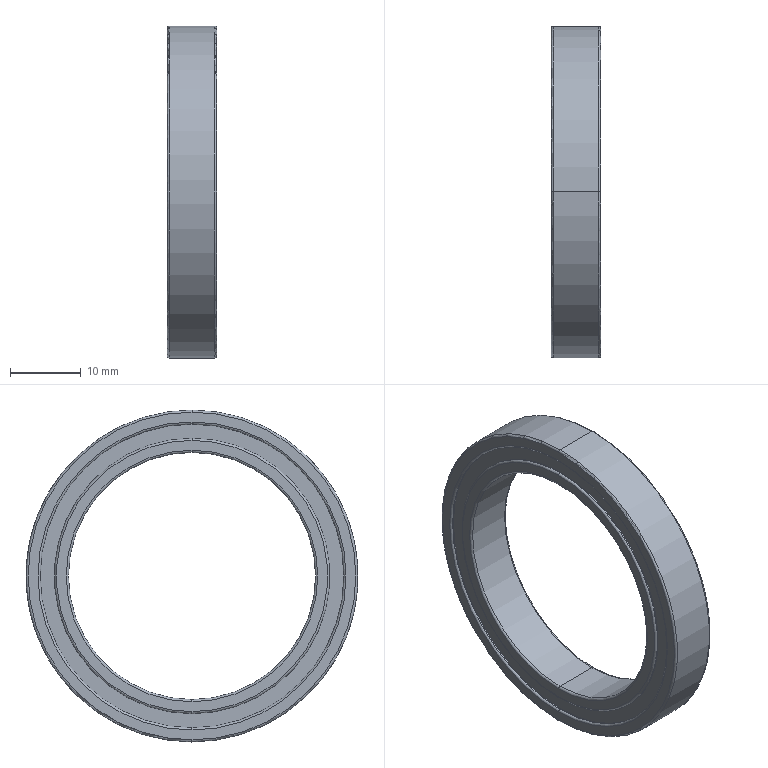Part | SolidWorks | features Revolution 5, CirPattern 2, RefAxis 1, RevCut 1 | 35 solids | 392 faces | box 7 x 47 x 47 mm | volume 4099 mm3 | cylinder 154 | sphere 140 | plane 76 | torus 22 | commonest cylinder face diameters 40.4 x67 41.6 x67 39 x8 43 x8 35 x2 47 x2